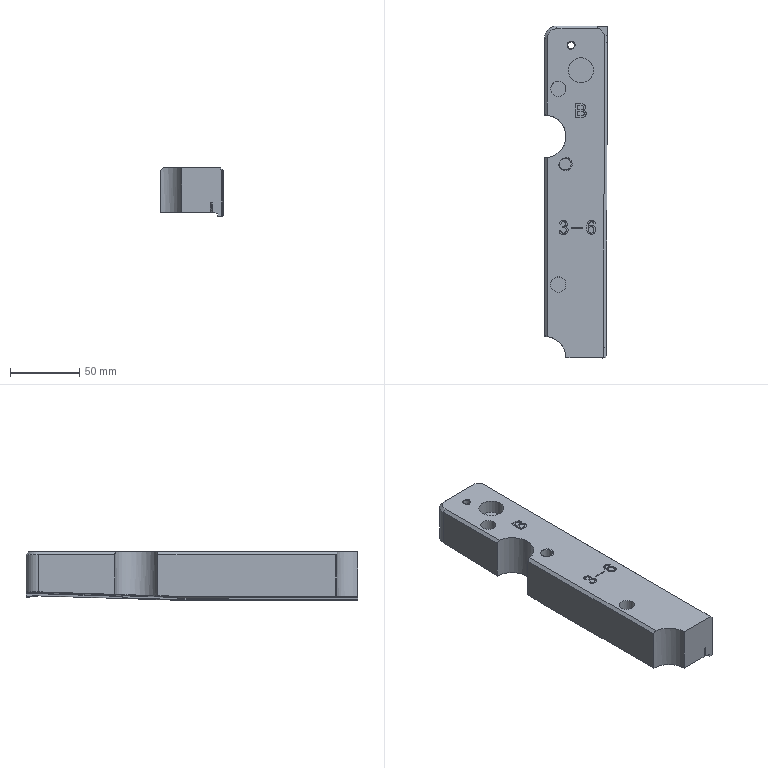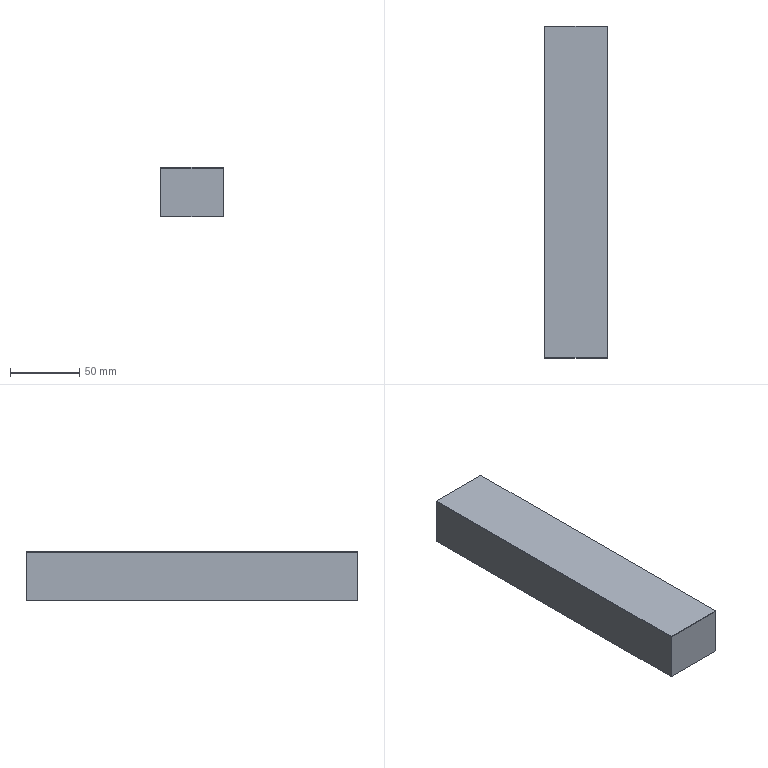CAM job | NX | 3-axis milling, drilling | part box 45.476 x 239.737 x 35.001 mm | stock box 45.476 x 239.737 x 35.501 mm
Tools:
number,name,description,diameter,corner_radius,flute_length,length,flutes
0,D16R0.8,Milling Tool-5 Parameters,16.0,0.8,50.0,75.0,2
0,D10,Milling Tool-5 Parameters,10.0,0.0,50.0,75.0,2
0,Z3,Drilling Tool,3.0,0.0,35.0,50.0,2
0,Z8.5,Drilling Tool,8.5,0.0,35.0,50.0,2
0,B1,Milling Tool-Ball Mill,1.0,0.5,50.0,75.0,2
0,D8,Milling Tool-5 Parameters,8.0,0.0,50.0,75.0,2
0,D8R0.5,Milling Tool-5 Parameters,8.0,0.5,50.0,75.0,2
Operations:
program,operation,operation_type,tool,method,geometry_group,spindle_rpm,surface_speed,feed_per_tooth,feed_cut,feed_plunge,cut_length_mm,path_length_mm,cut_time_min,machine_time_min
3-6,CAVITY_MILL_2,CavityMilling,D16R0.8,METHOD,WORKPIECE_2,2500.0,125.0,0.46,2300.0,60.0,26963.504,50775.109,12.457,15.2
3-6,HOLE_MILLING_1,CylinderMilling,D10,METHOD,WORKPIECE_2,3500.0,109.0,0.2143,1500.0,100.0,1864.128,1934.833,1.243,1.254
3-D10.NC_1,HOLE_MILLING_1_COPY,CylinderMilling,D10,METHOD,WORKPIECE_2,3500.0,109.0,0.2143,1500.0,100.0,1777.645,1847.552,1.185,1.197
3-D10.NC_1,ZLEVEL_PROFILE_2,ZLevelMilling,D10,METHOD,WORKPIECE_2,3470.0,109.0,0.2882,2000.0,100.0,1230.508,1295.708,0.6153,0.6263
3-6,SPOT_DRILLING_1,Operation,Z3,METHOD,WORKPIECE_2,3000.0,28.0,0.0083,50.0,0.0,8.0,253.497,0.16,0.1845
3-6,SPOT_DRILLING_1_COPY,Operation,Z8.5,METHOD,WORKPIECE_2,600.0,16.0,0.0417,50.0,0.0,93.0,389.862,1.86,1.89
3-6,PLANAR_TEXT_2,Engraving,B1,METHOD,WORKPIECE_2,7500.0,23.0,0.1,1500.0,50.0,742.902,1636.387,0.5129,0.6104
3-6,CAVITY_MILL_2_COPY_COPY,CavityMilling,D16R0.8,METHOD,WORKPIECE_2_COPY,2500.0,125.0,0.46,2300.0,60.0,103357.838,138362.103,46.772,50.766
3-6,CAVITY_MILL_2_COPY_COPY_COPY,CavityMilling,D8,METHOD,WORKPIECE_2_COPY,4500.0,125.0,0.46,2300.0,60.0,17008.19,28928.078,7.63,9.649
3-6Z,FACE_MILLING_COPY,FaceMilling,D8,METHOD,WORKPIECE_2_COPY,4500.0,113.0,0.1111,1000.0,60.0,2058.266,2763.792,2.075,2.171
3-6Z,ZLEVEL_PROFILE,ZLevelMilling,D8R0.5,METHOD,WORKPIECE_2_COPY,4500.0,113.0,0.2556,2300.0,60.0,70991.361,72189.698,32.283,32.428
3-6Z,ZLEVEL_PROFILE_COPY,ZLevelMilling,D8R0.5,METHOD,WORKPIECE_2_COPY,4500.0,113.0,0.2556,2300.0,60.0,4456.486,4508.905,1.994,2.003
3-6Z,ZLEVEL_PROFILE_COPY_COPY,ZLevelMilling,D8R0.5,METHOD,WORKPIECE_2_COPY,4500.0,113.0,0.2556,2300.0,60.0,47101.66,47554.23,21.619,21.678